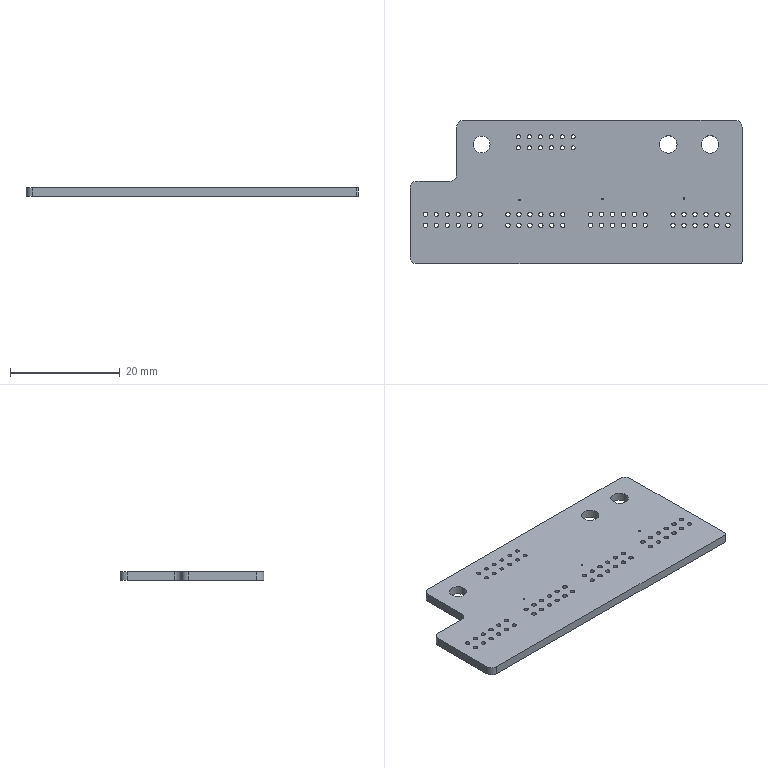Part | STEP file | Control module adapter PCB | 1 solid | 80 faces | box 60.512 x 26.172 x 1.6 mm | volume 2296 mm3 | cylinder 72 | plane 8 | commonest cylinder face diameters 0.8 x48 0.7 x12 2.54 x5 0.3 x3 3.2 x2 0.704 x1